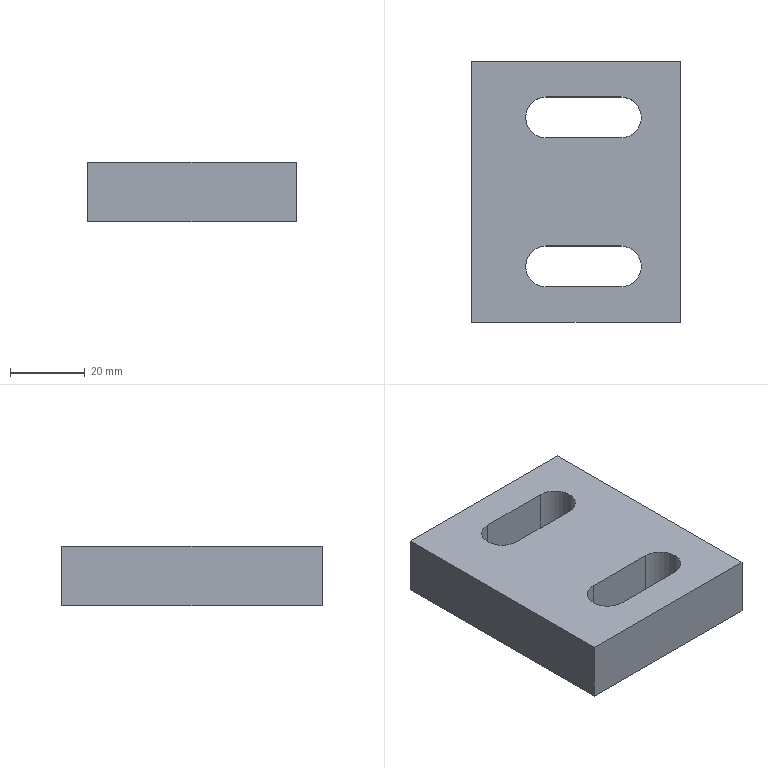Part | 1 solid | 16 faces | box 56 x 70 x 16 mm | volume 52639 mm3 | plane 10 | cylinder 6 | commonest cylinder face diameters 11 x6
STEP:
#1=CARTESIAN_POINT('',(-13.5,20.,16.));
#2=VERTEX_POINT('',#1);
#3=CARTESIAN_POINT('',(-8.,25.5,16.));
#4=VERTEX_POINT('',#3);
#5=CARTESIAN_POINT('',(-8.,20.,16.));
#6=DIRECTION('',(0.,0.,-1.));
#7=DIRECTION('',(-1.,0.,0.));
#8=AXIS2_PLACEMENT_3D('',#5,#6,#7);
#9=CIRCLE('',#8,5.5);
#10=EDGE_CURVE('',#2,#4,#9,.T.);
#11=ORIENTED_EDGE('',*,*,#10,.F.);
#12=CARTESIAN_POINT('',(-13.5,20.,0.));
#13=VERTEX_POINT('',#12);
#14=CARTESIAN_POINT('',(-13.5,20.,16.));
#15=DIRECTION('',(0.,0.,-1.));
#16=VECTOR('',#15,1000.);
#17=LINE('',#14,#16);
#18=EDGE_CURVE('',#2,#13,#17,.T.);
#19=ORIENTED_EDGE('',*,*,#18,.T.);
#20=CARTESIAN_POINT('',(-8.,25.5,0.));
#21=VERTEX_POINT('',#20);
#22=CARTESIAN_POINT('',(-8.,20.,0.));
#23=DIRECTION('',(0.,0.,1.));
#24=DIRECTION('',(-1.,0.,0.));
#25=AXIS2_PLACEMENT_3D('',#22,#23,#24);
#26=CIRCLE('',#25,5.5);
#27=EDGE_CURVE('',#21,#13,#26,.T.);
#28=ORIENTED_EDGE('',*,*,#27,.F.);
#29=CARTESIAN_POINT('',(-8.,25.5,16.));
#30=DIRECTION('',(0.,0.,-1.));
#31=VECTOR('',#30,1000.);
#32=LINE('',#29,#31);
#33=EDGE_CURVE('',#4,#21,#32,.T.);
#34=ORIENTED_EDGE('',*,*,#33,.F.);
#35=EDGE_LOOP('',(#11,#19,#28,#34));
#36=FACE_OUTER_BOUND('',#35,.T.);
#37=CARTESIAN_POINT('',(-8.,20.,16.));
#38=DIRECTION('',(0.,0.,-1.));
#39=DIRECTION('',(-1.,0.,0.));
#40=AXIS2_PLACEMENT_3D('',#37,#38,#39);
#41=CYLINDRICAL_SURFACE('',#40,5.5);
#42=ADVANCED_FACE('',(#36),#41,.F.);
#43=CARTESIAN_POINT('',(-13.5,-20.,16.));
#44=VERTEX_POINT('',#43);
#45=CARTESIAN_POINT('',(-8.,-14.5,16.));
#46=VERTEX_POINT('',#45);
#47=CARTESIAN_POINT('',(-8.,-20.,16.));
#48=DIRECTION('',(0.,0.,-1.));
#49=DIRECTION('',(1.,0.,0.));
#50=AXIS2_PLACEMENT_3D('',#47,#48,#49);
#51=CIRCLE('',#50,5.5);
#52=EDGE_CURVE('',#44,#46,#51,.T.);
#53=ORIENTED_EDGE('',*,*,#52,.F.);
#54=CARTESIAN_POINT('',(-13.5,-20.,0.));
#55=VERTEX_POINT('',#54);
#56=CARTESIAN_POINT('',(-13.5,-20.,16.));
#57=DIRECTION('',(0.,0.,-1.));
#58=VECTOR('',#57,1000.);
#59=LINE('',#56,#58);
#60=EDGE_CURVE('',#44,#55,#59,.T.);
#61=ORIENTED_EDGE('',*,*,#60,.T.);
#62=CARTESIAN_POINT('',(-8.,-14.5,0.));
#63=VERTEX_POINT('',#62);
#64=CARTESIAN_POINT('',(-8.,-20.,0.));
#65=DIRECTION('',(0.,0.,1.));
#66=DIRECTION('',(-1.,0.,0.));
#67=AXIS2_PLACEMENT_3D('',#64,#65,#66);
#68=CIRCLE('',#67,5.5);
#69=EDGE_CURVE('',#63,#55,#68,.T.);
#70=ORIENTED_EDGE('',*,*,#69,.F.);
#71=CARTESIAN_POINT('',(-8.,-14.5,16.));
#72=DIRECTION('',(0.,0.,-1.));
#73=VECTOR('',#72,1000.);
#74=LINE('',#71,#73);
#75=EDGE_CURVE('',#46,#63,#74,.T.);
#76=ORIENTED_EDGE('',*,*,#75,.F.);
#77=EDGE_LOOP('',(#53,#61,#70,#76));
#78=FACE_OUTER_BOUND('',#77,.T.);
#79=CARTESIAN_POINT('',(-8.,-20.,16.));
#80=DIRECTION('',(0.,0.,-1.));
#81=DIRECTION('',(-1.,0.,0.));
#82=AXIS2_PLACEMENT_3D('',#79,#80,#81);
#83=CYLINDRICAL_SURFACE('',#82,5.5);
#84=ADVANCED_FACE('',(#78),#83,.F.);
#85=CARTESIAN_POINT('',(28.,-35.,0.));
#86=VERTEX_POINT('',#85);
#87=CARTESIAN_POINT('',(28.,35.,0.));
#88=VERTEX_POINT('',#87);
#89=CARTESIAN_POINT('',(28.,35.,0.));
#90=DIRECTION('',(0.,1.,0.));
#91=VECTOR('',#90,1000.);
#92=LINE('',#89,#91);
#93=EDGE_CURVE('',#86,#88,#92,.T.);
#94=ORIENTED_EDGE('',*,*,#93,.T.);
#95=CARTESIAN_POINT('',(28.,35.,16.));
#96=VERTEX_POINT('',#95);
#97=CARTESIAN_POINT('',(28.,35.,16.));
#98=DIRECTION('',(0.,0.,-1.));
#99=VECTOR('',#98,1000.);
#100=LINE('',#97,#99);
#101=EDGE_CURVE('',#96,#88,#100,.T.);
#102=ORIENTED_EDGE('',*,*,#101,.F.);
#103=CARTESIAN_POINT('',(28.,-35.,16.));
#104=VERTEX_POINT('',#103);
#105=CARTESIAN_POINT('',(28.,35.,16.));
#106=DIRECTION('',(0.,1.,0.));
#107=VECTOR('',#106,1000.);
#108=LINE('',#105,#107);
#109=EDGE_CURVE('',#104,#96,#108,.T.);
#110=ORIENTED_EDGE('',*,*,#109,.F.);
#111=CARTESIAN_POINT('',(28.,-35.,16.));
#112=DIRECTION('',(0.,0.,-1.));
#113=VECTOR('',#112,1000.);
#114=LINE('',#111,#113);
#115=EDGE_CURVE('',#104,#86,#114,.T.);
#116=ORIENTED_EDGE('',*,*,#115,.T.);
#117=EDGE_LOOP('',(#94,#102,#110,#116));
#118=FACE_OUTER_BOUND('',#117,.T.);
#119=CARTESIAN_POINT('',(28.,35.,16.));
#120=DIRECTION('',(-1.,0.,0.));
#121=DIRECTION('',(0.,-1.,0.));
#122=AXIS2_PLACEMENT_3D('',#119,#120,#121);
#123=PLANE('',#122);
#124=ADVANCED_FACE('',(#118),#123,.F.);
#125=CARTESIAN_POINT('',(-28.,35.,0.));
#126=VERTEX_POINT('',#125);
#127=CARTESIAN_POINT('',(-28.,35.,0.));
#128=DIRECTION('',(-1.,0.,0.));
#129=VECTOR('',#128,1000.);
#130=LINE('',#127,#129);
#131=EDGE_CURVE('',#88,#126,#130,.T.);
#132=ORIENTED_EDGE('',*,*,#131,.T.);
#133=CARTESIAN_POINT('',(-28.,35.,16.));
#134=VERTEX_POINT('',#133);
#135=CARTESIAN_POINT('',(-28.,35.,16.));
#136=DIRECTION('',(0.,0.,-1.));
#137=VECTOR('',#136,1000.);
#138=LINE('',#135,#137);
#139=EDGE_CURVE('',#134,#126,#138,.T.);
#140=ORIENTED_EDGE('',*,*,#139,.F.);
#141=CARTESIAN_POINT('',(-28.,35.,16.));
#142=DIRECTION('',(-1.,0.,0.));
#143=VECTOR('',#142,1000.);
#144=LINE('',#141,#143);
#145=EDGE_CURVE('',#96,#134,#144,.T.);
#146=ORIENTED_EDGE('',*,*,#145,.F.);
#147=ORIENTED_EDGE('',*,*,#101,.T.);
#148=EDGE_LOOP('',(#132,#140,#146,#147));
#149=FACE_OUTER_BOUND('',#148,.T.);
#150=CARTESIAN_POINT('',(-28.,35.,16.));
#151=DIRECTION('',(0.,-1.,0.));
#152=DIRECTION('',(0.,0.,-1.));
#153=AXIS2_PLACEMENT_3D('',#150,#151,#152);
#154=PLANE('',#153);
#155=ADVANCED_FACE('',(#149),#154,.F.);
#156=CARTESIAN_POINT('',(-28.,-35.,0.));
#157=VERTEX_POINT('',#156);
#158=CARTESIAN_POINT('',(-28.,35.,0.));
#159=DIRECTION('',(0.,-1.,0.));
#160=VECTOR('',#159,1000.);
#161=LINE('',#158,#160);
#162=EDGE_CURVE('',#126,#157,#161,.T.);
#163=ORIENTED_EDGE('',*,*,#162,.T.);
#164=CARTESIAN_POINT('',(-28.,-35.,16.));
#165=VERTEX_POINT('',#164);
#166=CARTESIAN_POINT('',(-28.,-35.,16.));
#167=DIRECTION('',(0.,0.,-1.));
#168=VECTOR('',#167,1000.);
#169=LINE('',#166,#168);
#170=EDGE_CURVE('',#165,#157,#169,.T.);
#171=ORIENTED_EDGE('',*,*,#170,.F.);
#172=CARTESIAN_POINT('',(-28.,35.,16.));
#173=DIRECTION('',(0.,-1.,0.));
#174=VECTOR('',#173,1000.);
#175=LINE('',#172,#174);
#176=EDGE_CURVE('',#134,#165,#175,.T.);
#177=ORIENTED_EDGE('',*,*,#176,.F.);
#178=ORIENTED_EDGE('',*,*,#139,.T.);
#179=EDGE_LOOP('',(#163,#171,#177,#178));
#180=FACE_OUTER_BOUND('',#179,.T.);
#181=CARTESIAN_POINT('',(-28.,35.,16.));
#182=DIRECTION('',(1.,0.,0.));
#183=DIRECTION('',(0.,1.,0.));
#184=AXIS2_PLACEMENT_3D('',#181,#182,#183);
#185=PLANE('',#184);
#186=ADVANCED_FACE('',(#180),#185,.F.);
#187=CARTESIAN_POINT('',(-28.,-35.,0.));
#188=DIRECTION('',(1.,0.,0.));
#189=VECTOR('',#188,1000.);
#190=LINE('',#187,#189);
#191=EDGE_CURVE('',#157,#86,#190,.T.);
#192=ORIENTED_EDGE('',*,*,#191,.T.);
#193=ORIENTED_EDGE('',*,*,#115,.F.);
#194=CARTESIAN_POINT('',(-28.,-35.,16.));
#195=DIRECTION('',(1.,0.,0.));
#196=VECTOR('',#195,1000.);
#197=LINE('',#194,#196);
#198=EDGE_CURVE('',#165,#104,#197,.T.);
#199=ORIENTED_EDGE('',*,*,#198,.F.);
#200=ORIENTED_EDGE('',*,*,#170,.T.);
#201=EDGE_LOOP('',(#192,#193,#199,#200));
#202=FACE_OUTER_BOUND('',#201,.T.);
#203=CARTESIAN_POINT('',(-28.,-35.,16.));
#204=DIRECTION('',(0.,1.,0.));
#205=DIRECTION('',(0.,0.,1.));
#206=AXIS2_PLACEMENT_3D('',#203,#204,#205);
#207=PLANE('',#206);
#208=ADVANCED_FACE('',(#202),#207,.F.);
#209=CARTESIAN_POINT('',(12.,25.5,16.));
#210=VERTEX_POINT('',#209);
#211=CARTESIAN_POINT('',(12.,14.5,16.));
#212=VERTEX_POINT('',#211);
#213=CARTESIAN_POINT('',(12.,20.,16.));
#214=DIRECTION('',(0.,0.,-1.));
#215=DIRECTION('',(-1.,0.,0.));
#216=AXIS2_PLACEMENT_3D('',#213,#214,#215);
#217=CIRCLE('',#216,5.5);
#218=EDGE_CURVE('',#210,#212,#217,.T.);
#219=ORIENTED_EDGE('',*,*,#218,.T.);
#220=CARTESIAN_POINT('',(-8.,14.5,16.));
#221=VERTEX_POINT('',#220);
#222=CARTESIAN_POINT('',(12.,14.5,16.));
#223=DIRECTION('',(-1.,0.,0.));
#224=VECTOR('',#223,1000.);
#225=LINE('',#222,#224);
#226=EDGE_CURVE('',#212,#221,#225,.T.);
#227=ORIENTED_EDGE('',*,*,#226,.T.);
#228=CARTESIAN_POINT('',(-8.,20.,16.));
#229=DIRECTION('',(0.,0.,-1.));
#230=DIRECTION('',(-1.,0.,0.));
#231=AXIS2_PLACEMENT_3D('',#228,#229,#230);
#232=CIRCLE('',#231,5.5);
#233=EDGE_CURVE('',#221,#2,#232,.T.);
#234=ORIENTED_EDGE('',*,*,#233,.T.);
#235=ORIENTED_EDGE('',*,*,#10,.T.);
#236=CARTESIAN_POINT('',(12.,25.5,16.));
#237=DIRECTION('',(1.,0.,0.));
#238=VECTOR('',#237,1000.);
#239=LINE('',#236,#238);
#240=EDGE_CURVE('',#4,#210,#239,.T.);
#241=ORIENTED_EDGE('',*,*,#240,.T.);
#242=EDGE_LOOP('',(#219,#227,#234,#235,#241));
#243=FACE_BOUND('',#242,.T.);
#244=CARTESIAN_POINT('',(12.,-14.5,16.));
#245=VERTEX_POINT('',#244);
#246=CARTESIAN_POINT('',(12.,-25.5,16.));
#247=VERTEX_POINT('',#246);
#248=CARTESIAN_POINT('',(12.,-20.,16.));
#249=DIRECTION('',(0.,0.,-1.));
#250=DIRECTION('',(1.,0.,0.));
#251=AXIS2_PLACEMENT_3D('',#248,#249,#250);
#252=CIRCLE('',#251,5.5);
#253=EDGE_CURVE('',#245,#247,#252,.T.);
#254=ORIENTED_EDGE('',*,*,#253,.T.);
#255=CARTESIAN_POINT('',(-8.,-25.5,16.));
#256=VERTEX_POINT('',#255);
#257=CARTESIAN_POINT('',(12.,-25.5,16.));
#258=DIRECTION('',(-1.,0.,0.));
#259=VECTOR('',#258,1000.);
#260=LINE('',#257,#259);
#261=EDGE_CURVE('',#247,#256,#260,.T.);
#262=ORIENTED_EDGE('',*,*,#261,.T.);
#263=CARTESIAN_POINT('',(-8.,-20.,16.));
#264=DIRECTION('',(0.,0.,-1.));
#265=DIRECTION('',(1.,0.,0.));
#266=AXIS2_PLACEMENT_3D('',#263,#264,#265);
#267=CIRCLE('',#266,5.5);
#268=EDGE_CURVE('',#256,#44,#267,.T.);
#269=ORIENTED_EDGE('',*,*,#268,.T.);
#270=ORIENTED_EDGE('',*,*,#52,.T.);
#271=CARTESIAN_POINT('',(12.,-14.5,16.));
#272=DIRECTION('',(1.,0.,0.));
#273=VECTOR('',#272,1000.);
#274=LINE('',#271,#273);
#275=EDGE_CURVE('',#46,#245,#274,.T.);
#276=ORIENTED_EDGE('',*,*,#275,.T.);
#277=EDGE_LOOP('',(#254,#262,#269,#270,#276));
#278=FACE_BOUND('',#277,.T.);
#279=ORIENTED_EDGE('',*,*,#109,.T.);
#280=ORIENTED_EDGE('',*,*,#145,.T.);
#281=ORIENTED_EDGE('',*,*,#176,.T.);
#282=ORIENTED_EDGE('',*,*,#198,.T.);
#283=EDGE_LOOP('',(#279,#280,#281,#282));
#284=FACE_OUTER_BOUND('',#283,.T.);
#285=CARTESIAN_POINT('',(0.,0.,16.));
#286=DIRECTION('',(0.,0.,1.));
#287=DIRECTION('',(1.,0.,0.));
#288=AXIS2_PLACEMENT_3D('',#285,#286,#287);
#289=PLANE('',#288);
#290=ADVANCED_FACE('',(#243,#278,#284),#289,.T.);
#291=CARTESIAN_POINT('',(-8.,14.5,0.));
#292=VERTEX_POINT('',#291);
#293=CARTESIAN_POINT('',(12.,14.5,0.));
#294=VERTEX_POINT('',#293);
#295=CARTESIAN_POINT('',(0.,14.5,0.));
#296=DIRECTION('',(1.,0.,0.));
#297=VECTOR('',#296,1000.);
#298=LINE('',#295,#297);
#299=EDGE_CURVE('',#292,#294,#298,.T.);
#300=ORIENTED_EDGE('',*,*,#299,.T.);
#301=CARTESIAN_POINT('',(12.,25.5,0.));
#302=VERTEX_POINT('',#301);
#303=CARTESIAN_POINT('',(12.,20.,0.));
#304=DIRECTION('',(0.,0.,1.));
#305=DIRECTION('',(-1.,0.,0.));
#306=AXIS2_PLACEMENT_3D('',#303,#304,#305);
#307=CIRCLE('',#306,5.5);
#308=EDGE_CURVE('',#294,#302,#307,.T.);
#309=ORIENTED_EDGE('',*,*,#308,.T.);
#310=CARTESIAN_POINT('',(0.,25.5,0.));
#311=DIRECTION('',(-1.,0.,0.));
#312=VECTOR('',#311,1000.);
#313=LINE('',#310,#312);
#314=EDGE_CURVE('',#302,#21,#313,.T.);
#315=ORIENTED_EDGE('',*,*,#314,.T.);
#316=ORIENTED_EDGE('',*,*,#27,.T.);
#317=CARTESIAN_POINT('',(-8.,20.,0.));
#318=DIRECTION('',(0.,0.,1.));
#319=DIRECTION('',(-1.,0.,0.));
#320=AXIS2_PLACEMENT_3D('',#317,#318,#319);
#321=CIRCLE('',#320,5.5);
#322=EDGE_CURVE('',#13,#292,#321,.T.);
#323=ORIENTED_EDGE('',*,*,#322,.T.);
#324=EDGE_LOOP('',(#300,#309,#315,#316,#323));
#325=FACE_BOUND('',#324,.T.);
#326=CARTESIAN_POINT('',(-8.,-25.5,0.));
#327=VERTEX_POINT('',#326);
#328=CARTESIAN_POINT('',(12.,-25.5,0.));
#329=VERTEX_POINT('',#328);
#330=CARTESIAN_POINT('',(0.,-25.5,0.));
#331=DIRECTION('',(1.,0.,0.));
#332=VECTOR('',#331,1000.);
#333=LINE('',#330,#332);
#334=EDGE_CURVE('',#327,#329,#333,.T.);
#335=ORIENTED_EDGE('',*,*,#334,.T.);
#336=CARTESIAN_POINT('',(12.,-14.5,0.));
#337=VERTEX_POINT('',#336);
#338=CARTESIAN_POINT('',(12.,-20.,0.));
#339=DIRECTION('',(0.,0.,1.));
#340=DIRECTION('',(-1.,0.,0.));
#341=AXIS2_PLACEMENT_3D('',#338,#339,#340);
#342=CIRCLE('',#341,5.5);
#343=EDGE_CURVE('',#329,#337,#342,.T.);
#344=ORIENTED_EDGE('',*,*,#343,.T.);
#345=CARTESIAN_POINT('',(0.,-14.5,0.));
#346=DIRECTION('',(-1.,0.,0.));
#347=VECTOR('',#346,1000.);
#348=LINE('',#345,#347);
#349=EDGE_CURVE('',#337,#63,#348,.T.);
#350=ORIENTED_EDGE('',*,*,#349,.T.);
#351=ORIENTED_EDGE('',*,*,#69,.T.);
#352=CARTESIAN_POINT('',(-8.,-20.,0.));
#353=DIRECTION('',(0.,0.,1.));
#354=DIRECTION('',(-1.,0.,0.));
#355=AXIS2_PLACEMENT_3D('',#352,#353,#354);
#356=CIRCLE('',#355,5.5);
#357=EDGE_CURVE('',#55,#327,#356,.T.);
#358=ORIENTED_EDGE('',*,*,#357,.T.);
#359=EDGE_LOOP('',(#335,#344,#350,#351,#358));
#360=FACE_BOUND('',#359,.T.);
#361=ORIENTED_EDGE('',*,*,#93,.F.);
#362=ORIENTED_EDGE('',*,*,#191,.F.);
#363=ORIENTED_EDGE('',*,*,#162,.F.);
#364=ORIENTED_EDGE('',*,*,#131,.F.);
#365=EDGE_LOOP('',(#361,#362,#363,#364));
#366=FACE_OUTER_BOUND('',#365,.T.);
#367=CARTESIAN_POINT('',(0.,0.,0.));
#368=DIRECTION('',(0.,0.,1.));
#369=DIRECTION('',(1.,0.,0.));
#370=AXIS2_PLACEMENT_3D('',#367,#368,#369);
#371=PLANE('',#370);
#372=ADVANCED_FACE('',(#325,#360,#366),#371,.F.);
#373=CARTESIAN_POINT('',(12.,-25.5,16.));
#374=DIRECTION('',(0.,0.,-1.));
#375=VECTOR('',#374,1000.);
#376=LINE('',#373,#375);
#377=EDGE_CURVE('',#247,#329,#376,.T.);
#378=ORIENTED_EDGE('',*,*,#377,.F.);
#379=ORIENTED_EDGE('',*,*,#253,.F.);
#380=CARTESIAN_POINT('',(12.,-14.5,16.));
#381=DIRECTION('',(0.,0.,-1.));
#382=VECTOR('',#381,1000.);
#383=LINE('',#380,#382);
#384=EDGE_CURVE('',#245,#337,#383,.T.);
#385=ORIENTED_EDGE('',*,*,#384,.T.);
#386=ORIENTED_EDGE('',*,*,#343,.F.);
#387=EDGE_LOOP('',(#378,#379,#385,#386));
#388=FACE_OUTER_BOUND('',#387,.T.);
#389=CARTESIAN_POINT('',(12.,-20.,16.));
#390=DIRECTION('',(0.,0.,-1.));
#391=DIRECTION('',(-1.,0.,0.));
#392=AXIS2_PLACEMENT_3D('',#389,#390,#391);
#393=CYLINDRICAL_SURFACE('',#392,5.5);
#394=ADVANCED_FACE('',(#388),#393,.F.);
#395=ORIENTED_EDGE('',*,*,#384,.F.);
#396=ORIENTED_EDGE('',*,*,#275,.F.);
#397=ORIENTED_EDGE('',*,*,#75,.T.);
#398=ORIENTED_EDGE('',*,*,#349,.F.);
#399=EDGE_LOOP('',(#395,#396,#397,#398));
#400=FACE_OUTER_BOUND('',#399,.T.);
#401=CARTESIAN_POINT('',(12.,-14.5,16.));
#402=DIRECTION('',(0.,1.,0.));
#403=DIRECTION('',(-1.,0.,0.));
#404=AXIS2_PLACEMENT_3D('',#401,#402,#403);
#405=PLANE('',#404);
#406=ADVANCED_FACE('',(#400),#405,.F.);
#407=ORIENTED_EDGE('',*,*,#60,.F.);
#408=ORIENTED_EDGE('',*,*,#268,.F.);
#409=CARTESIAN_POINT('',(-8.,-25.5,16.));
#410=DIRECTION('',(0.,0.,-1.));
#411=VECTOR('',#410,1000.);
#412=LINE('',#409,#411);
#413=EDGE_CURVE('',#256,#327,#412,.T.);
#414=ORIENTED_EDGE('',*,*,#413,.T.);
#415=ORIENTED_EDGE('',*,*,#357,.F.);
#416=EDGE_LOOP('',(#407,#408,#414,#415));
#417=FACE_OUTER_BOUND('',#416,.T.);
#418=CARTESIAN_POINT('',(-8.,-20.,16.));
#419=DIRECTION('',(0.,0.,-1.));
#420=DIRECTION('',(-1.,0.,0.));
#421=AXIS2_PLACEMENT_3D('',#418,#419,#420);
#422=CYLINDRICAL_SURFACE('',#421,5.5);
#423=ADVANCED_FACE('',(#417),#422,.F.);
#424=ORIENTED_EDGE('',*,*,#413,.F.);
#425=ORIENTED_EDGE('',*,*,#261,.F.);
#426=ORIENTED_EDGE('',*,*,#377,.T.);
#427=ORIENTED_EDGE('',*,*,#334,.F.);
#428=EDGE_LOOP('',(#424,#425,#426,#427));
#429=FACE_OUTER_BOUND('',#428,.T.);
#430=CARTESIAN_POINT('',(12.,-25.5,16.));
#431=DIRECTION('',(0.,-1.,0.));
#432=DIRECTION('',(1.,0.,0.));
#433=AXIS2_PLACEMENT_3D('',#430,#431,#432);
#434=PLANE('',#433);
#435=ADVANCED_FACE('',(#429),#434,.F.);
#436=CARTESIAN_POINT('',(12.,14.5,16.));
#437=DIRECTION('',(0.,0.,-1.));
#438=VECTOR('',#437,1000.);
#439=LINE('',#436,#438);
#440=EDGE_CURVE('',#212,#294,#439,.T.);
#441=ORIENTED_EDGE('',*,*,#440,.F.);
#442=ORIENTED_EDGE('',*,*,#218,.F.);
#443=CARTESIAN_POINT('',(12.,25.5,16.));
#444=DIRECTION('',(0.,0.,-1.));
#445=VECTOR('',#444,1000.);
#446=LINE('',#443,#445);
#447=EDGE_CURVE('',#210,#302,#446,.T.);
#448=ORIENTED_EDGE('',*,*,#447,.T.);
#449=ORIENTED_EDGE('',*,*,#308,.F.);
#450=EDGE_LOOP('',(#441,#442,#448,#449));
#451=FACE_OUTER_BOUND('',#450,.T.);
#452=CARTESIAN_POINT('',(12.,20.,16.));
#453=DIRECTION('',(0.,0.,-1.));
#454=DIRECTION('',(-1.,0.,0.));
#455=AXIS2_PLACEMENT_3D('',#452,#453,#454);
#456=CYLINDRICAL_SURFACE('',#455,5.5);
#457=ADVANCED_FACE('',(#451),#456,.F.);
#458=ORIENTED_EDGE('',*,*,#447,.F.);
#459=ORIENTED_EDGE('',*,*,#240,.F.);
#460=ORIENTED_EDGE('',*,*,#33,.T.);
#461=ORIENTED_EDGE('',*,*,#314,.F.);
#462=EDGE_LOOP('',(#458,#459,#460,#461));
#463=FACE_OUTER_BOUND('',#462,.T.);
#464=CARTESIAN_POINT('',(12.,25.5,16.));
#465=DIRECTION('',(0.,1.,0.));
#466=DIRECTION('',(-1.,0.,0.));
#467=AXIS2_PLACEMENT_3D('',#464,#465,#466);
#468=PLANE('',#467);
#469=ADVANCED_FACE('',(#463),#468,.F.);
#470=ORIENTED_EDGE('',*,*,#18,.F.);
#471=ORIENTED_EDGE('',*,*,#233,.F.);
#472=CARTESIAN_POINT('',(-8.,14.5,16.));
#473=DIRECTION('',(0.,0.,-1.));
#474=VECTOR('',#473,1000.);
#475=LINE('',#472,#474);
#476=EDGE_CURVE('',#221,#292,#475,.T.);
#477=ORIENTED_EDGE('',*,*,#476,.T.);
#478=ORIENTED_EDGE('',*,*,#322,.F.);
#479=EDGE_LOOP('',(#470,#471,#477,#478));
#480=FACE_OUTER_BOUND('',#479,.T.);
#481=CARTESIAN_POINT('',(-8.,20.,16.));
#482=DIRECTION('',(0.,0.,-1.));
#483=DIRECTION('',(-1.,0.,0.));
#484=AXIS2_PLACEMENT_3D('',#481,#482,#483);
#485=CYLINDRICAL_SURFACE('',#484,5.5);
#486=ADVANCED_FACE('',(#480),#485,.F.);
#487=ORIENTED_EDGE('',*,*,#476,.F.);
#488=ORIENTED_EDGE('',*,*,#226,.F.);
#489=ORIENTED_EDGE('',*,*,#440,.T.);
#490=ORIENTED_EDGE('',*,*,#299,.F.);
#491=EDGE_LOOP('',(#487,#488,#489,#490));
#492=FACE_OUTER_BOUND('',#491,.T.);
#493=CARTESIAN_POINT('',(12.,14.5,16.));
#494=DIRECTION('',(0.,-1.,0.));
#495=DIRECTION('',(1.,0.,0.));
#496=AXIS2_PLACEMENT_3D('',#493,#494,#495);
#497=PLANE('',#496);
#498=ADVANCED_FACE('',(#492),#497,.F.);
#499=CLOSED_SHELL('',(#42,#84,#124,#155,#186,#208,#290,#372,#394,#406,#423,#435,#457,#469,#486,#498));
#500=MANIFOLD_SOLID_BREP('',#499);
#501=CARTESIAN_POINT('',(0.,0.,0.));
#502=DIRECTION('',(0.,0.,1.));
#503=DIRECTION('',(1.,0.,0.));
#504=AXIS2_PLACEMENT_3D('',#501,#502,#503);
#505=(LENGTH_UNIT()NAMED_UNIT(*)SI_UNIT(.MILLI.,.METRE.));
#506=UNCERTAINTY_MEASURE_WITH_UNIT(LENGTH_MEASURE(0.00001),#505,'','');
#507=(NAMED_UNIT(*)PLANE_ANGLE_UNIT()SI_UNIT($,.RADIAN.));
#508=(NAMED_UNIT(*)SI_UNIT($,.STERADIAN.)SOLID_ANGLE_UNIT());
#509=(GEOMETRIC_REPRESENTATION_CONTEXT(3)GLOBAL_UNCERTAINTY_ASSIGNED_CONTEXT((#506))GLOBAL_UNIT_ASSIGNED_CONTEXT((#505,#507,#508))REPRESENTATION_CONTEXT('',''));
#510=ADVANCED_BREP_SHAPE_REPRESENTATION('',(#500,#504),#509);